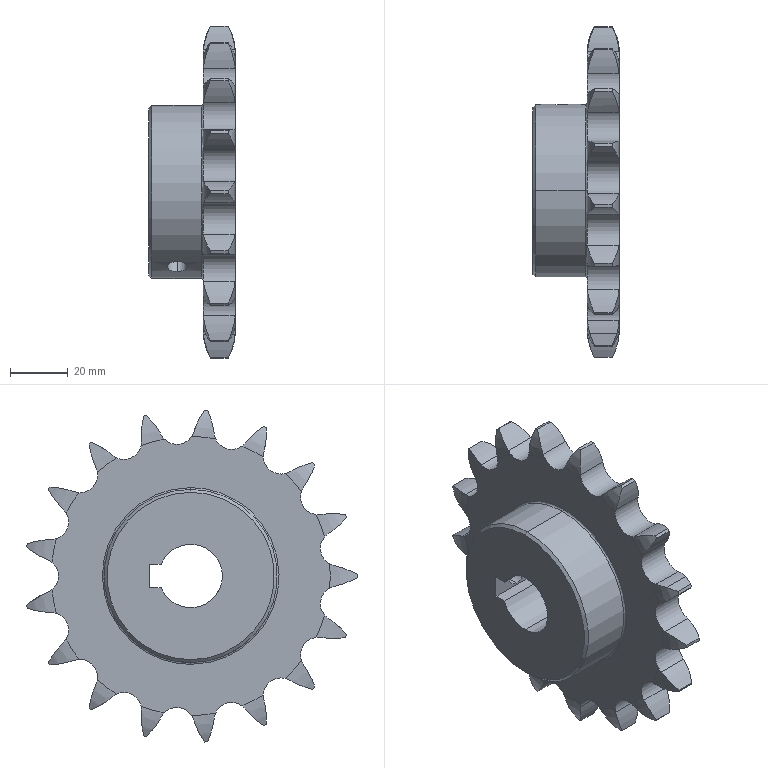Part | SolidWorks | features BaseBody 1, Chamfer 1, CirPattern 1, HoleWzd 1 | 1 solid | 128 faces | box 30.001 x 114.527 x 115.015 mm | volume 126258 mm3 | cylinder 84 | spline 36 | plane 6 | cone 2 | commonest cylinder face diameters 55.039 x35 12.191 x23 115.416 x17 6.8 x4 22 x3 60 x2